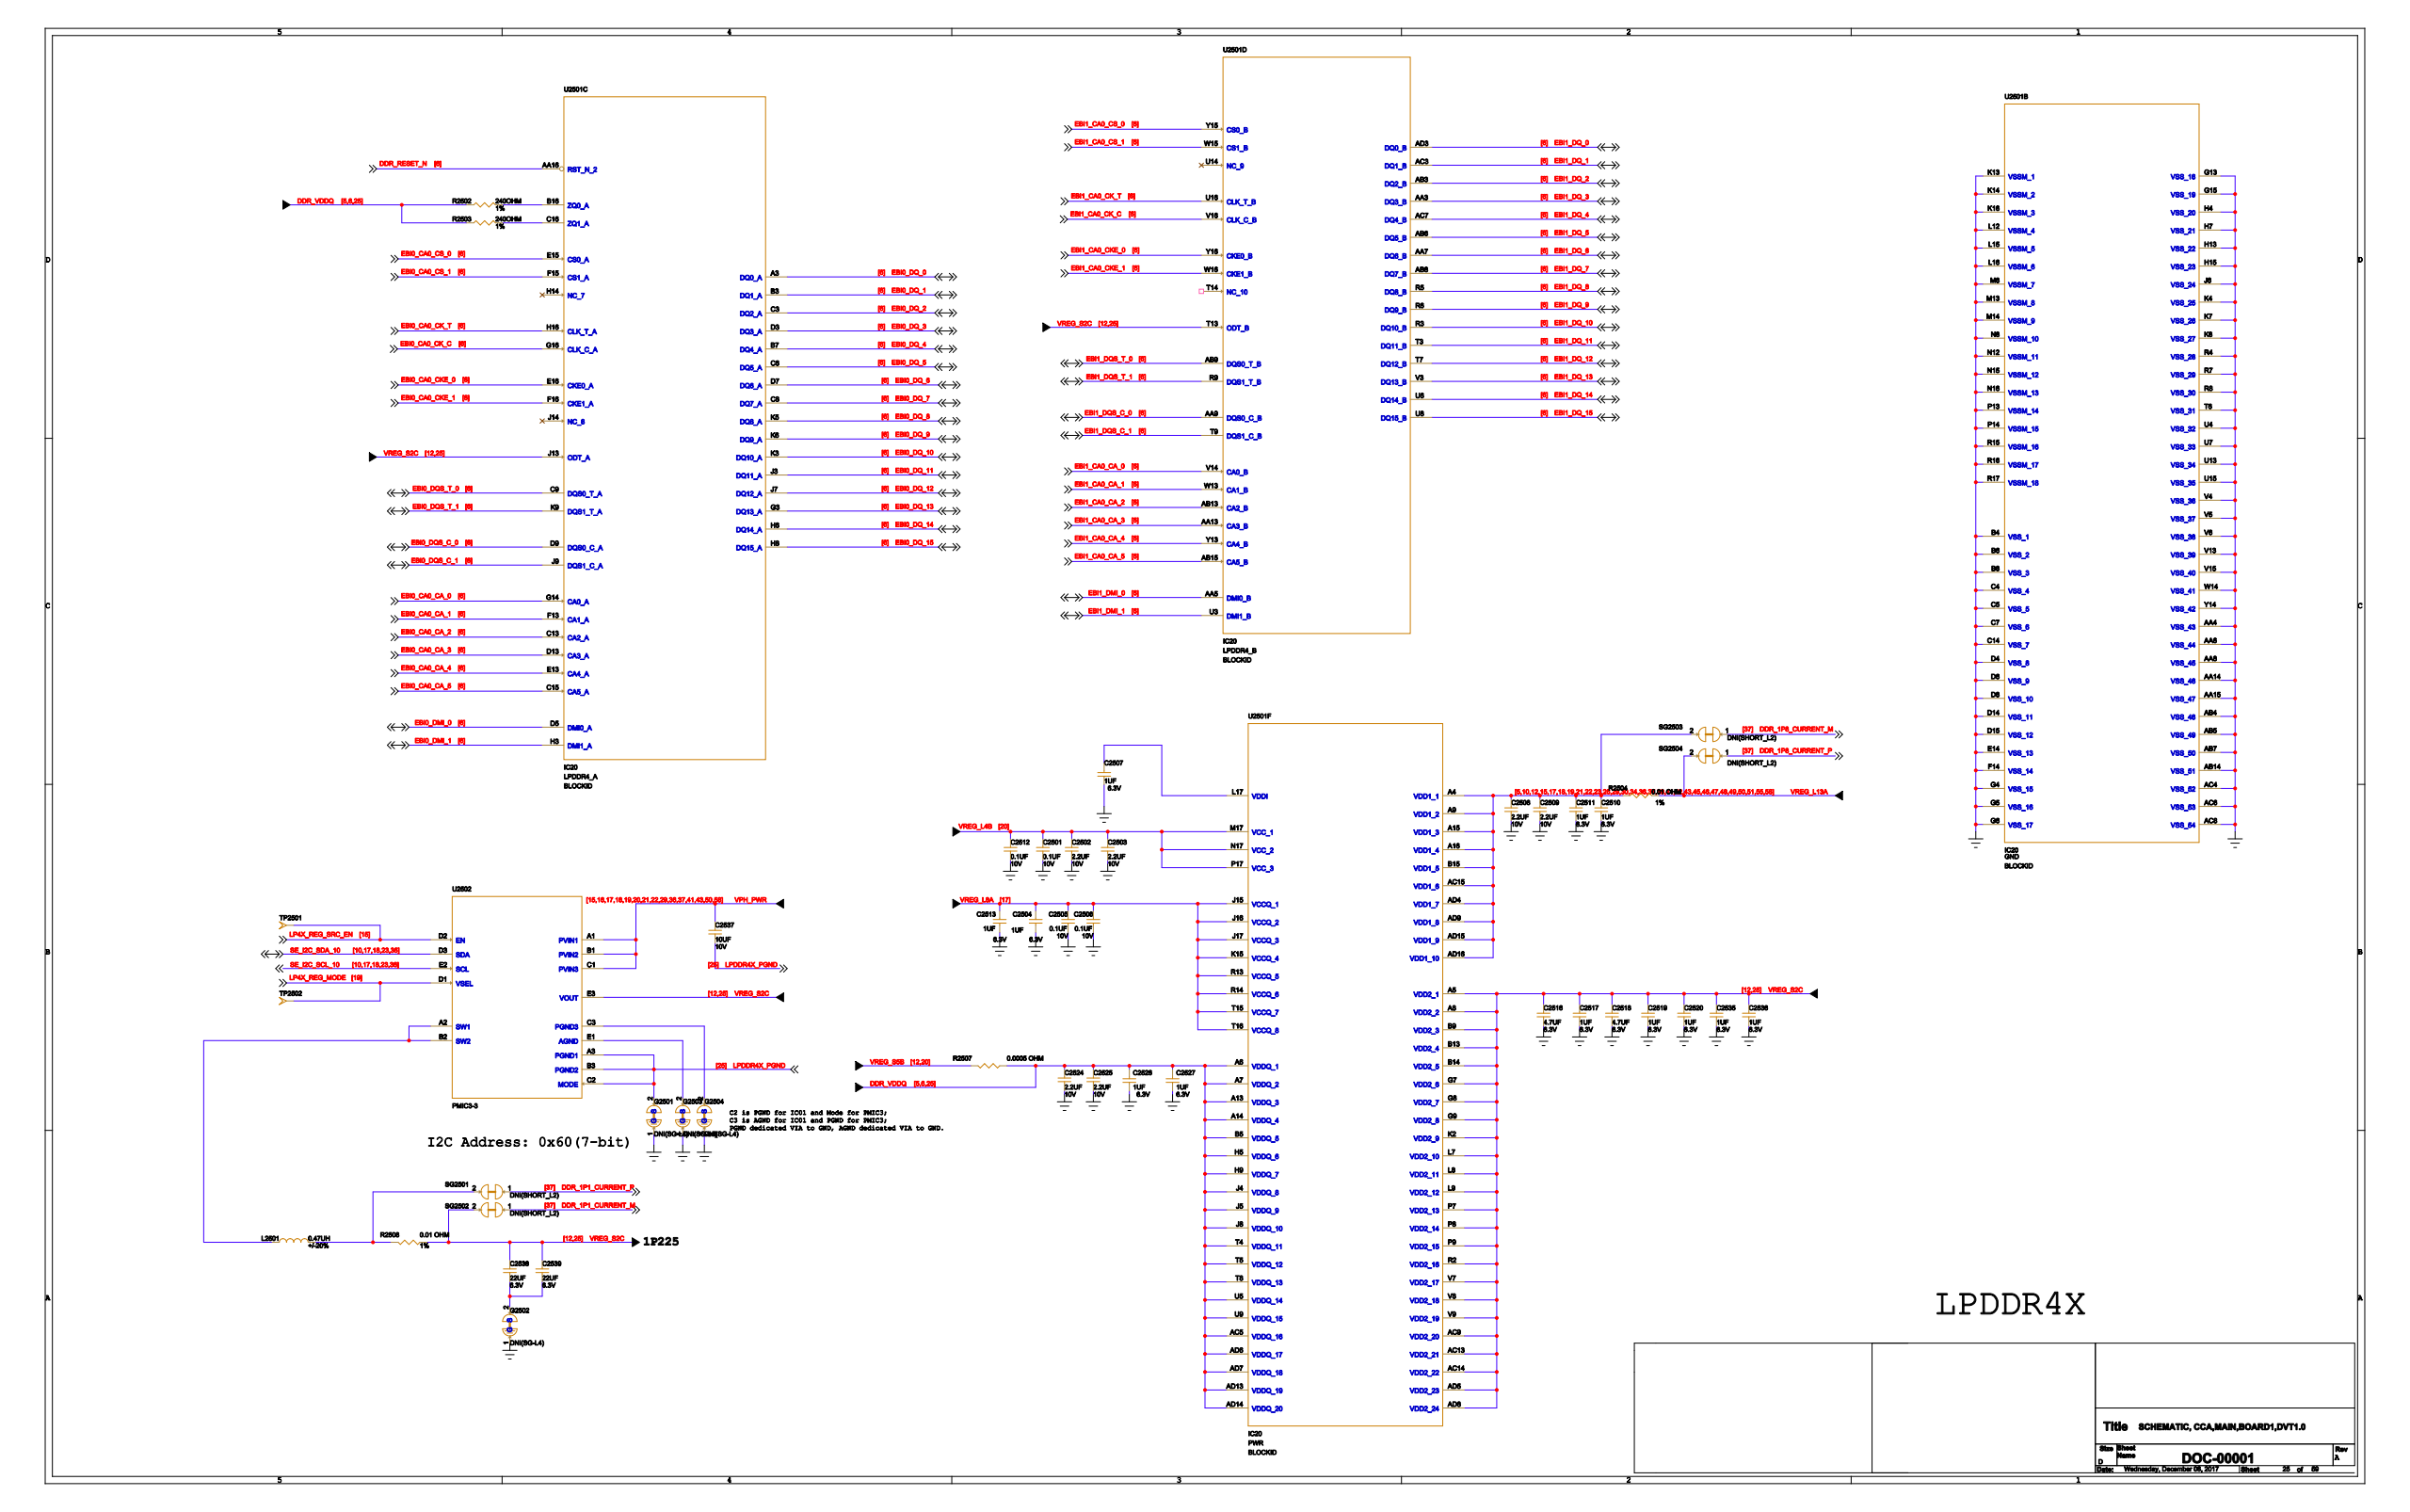Circuit board | KiCad | 1657 parts | 1365 nets | one sheet of the schematic
Parts on this sheet (reference | value | footprint):
C2501
C2502
C2503
C2504
C2505
C2506
C2507
C2508
C2509
C2510
C2511
C2512
C2513
C2516
C2517
C2518
C2519
C2520
C2524
C2525
C2526
C2527
C2535
C2536
C2537
C2538
C2539
G2501
G2502
G2503
G2504
L2501
R2502
R2503
R2504
R2507
R2508
SG2501
SG2502
SG2503
SG2504
TP2501
TP2502
U2501
U2502
Nets of these parts (net: part-pin ...):
DDR_VDDQ: C2524-1 C2525-1 C2526-2 C2527-2 R2502-1 R2503-1 R2507-2 U2501-A6 U2501-A7 U2501-A13 U2501-A14 U2501-AC5 U2501-AD6 U2501-AD7 U2501-AD13 U2501-AD14 U2501-B5 U2501-H5 U2501-H9 U2501-J4 U2501-J5 U2501-J8 U2501-T4 U2501-T5 U2501-T8 U2501-U5 U2501-U9
GND: C2501-2 C2502-2 C2503-2 C2504-2 C2505-2 C2506-2 C2507-1 C2508-2 C2509-2 C2510-2 C2511-2 C2512-2 C2513-2 C2516-2 C2517-2 C2518-2 C2519-2 C2520-2 C2524-2 C2525-2 C2526-1 C2527-1 C2535-2 C2536-2 G2501-1 G2502-1 G2503-1 G2504-1 U2501-AA4 U2501-AA6 U2501-AA8 U2501-AA14 U2501-AA15 U2501-AB4 U2501-AB5 U2501-AB7 U2501-AB14 U2501-AC4 U2501-AC6 U2501-AC8 U2501-B4 U2501-B6 U2501-B8 U2501-C4 U2501-C5 U2501-C7 U2501-C14 U2501-D4 U2501-D6 U2501-D8 U2501-D14 U2501-D15 U2501-E14 U2501-F14 U2501-G4 U2501-G5 U2501-G6 U2501-G13 U2501-G15 U2501-H4 U2501-H7 U2501-H13 U2501-H15 U2501-J6 U2501-K4 U2501-K7 U2501-K8 U2501-K13 U2501-K14 U2501-K16 U2501-L12 U2501-L15 U2501-L16 U2501-M8 U2501-M13 U2501-M14 U2501-N8 U2501-N12 U2501-N15 U2501-N16 U2501-P13 U2501-P14 U2501-R4 U2501-R7 U2501-R8 U2501-R15 U2501-R16 U2501-R17 U2501-T6 U2501-U4 U2501-U7 U2501-U13 U2501-U15 U2501-V4 U2501-V5 U2501-V6 U2501-V13 U2501-V15 U2501-W14 U2501-Y14
VREG_L13A: R2504-1 SG2504-2
VPH_PWR: C2537-1 U2502-A1 U2502-B1 U2502-C1
N23907455: C2508-1 C2509-1 C2510-1 C2511-1 R2504-2 SG2503-2 U2501-A4 U2501-A9 U2501-A15 U2501-A16 U2501-AC15 U2501-AD4 U2501-AD9 U2501-AD15 U2501-AD16 U2501-B15
SE_I2C_SCL_10: U2502-E2
SE_I2C_SDA_10: U2502-D3
VREG_S2C: C2516-1 C2517-1 C2518-1 C2519-1 C2520-1 C2535-1 C2536-1 C2538-1 C2539-1 R2508-2 SG2502-2 U2502-E3 U2501-A5 U2501-A8 U2501-AC9 U2501-AC13 U2501-AC14 U2501-AD5 U2501-AD8 U2501-B9 U2501-B13 U2501-B14 U2501-G7 U2501-G8 U2501-G9 U2501-J13 U2501-K2 U2501-L7 U2501-L8 U2501-L9 U2501-P7 U2501-P8 U2501-P9 U2501-R2 U2501-T13 U2501-V7 U2501-V8 U2501-V9
N23906069: R2503-2 U2501-C16
N23911865: C2538-2 C2539-2 G2502-2
_1P1_CURRENT_M: SG2502-1
N23907588: C2507-2 U2501-L17
N23911869: L2501-2 R2508-1 SG2501-2
N23907573: L2501-1 U2502-A2 U2502-B2
LPDDR4X_PGND: C2537-2 G2501-2 U2502-A3 U2502-B3 U2502-C2
N23907567: G2504-2 U2502-C3
LP4X_REG_MODE: TP2502-1 U2502-D1
P4X_REG_SRC_EN: TP2501-1 U2502-D2
N23907547: G2503-2 U2502-E1
VREG_L8A: C2504-1 C2505-1 C2506-1 C2513-1 U2501-J15 U2501-J16 U2501-J17 U2501-K15 U2501-R13 U2501-R14 U2501-T15 U2501-T16
EBI0_DQ_0: U2501-A3
EBI1_DQ_3: U2501-AA3
EBI1_DMI_0: U2501-AA5
EBI1_DQ_6: U2501-AA7
EBI1_DQS_C_0: U2501-AA9
EBI1_CA0_CA_3: U2501-AA13
DDR_RESET_N: U2501-AA16
EBI1_DQ_2: U2501-AB3
EBI1_DQ_5: U2501-AB6
EBI1_DQ_7: U2501-AB8
EBI1_DQS_T_0: U2501-AB9
EBI1_CA0_CA_2: U2501-AB13
EBI1_CA0_CA_5: U2501-AB15
EBI1_DQ_1: U2501-AC3
EBI1_DQ_4: U2501-AC7
EBI1_DQ_0: U2501-AD3
EBI0_DQ_1: U2501-B3
EBI0_DQ_4: U2501-B7
N23906067: R2502-2 U2501-B16
EBI0_DQ_2: U2501-C3
EBI0_DQ_5: U2501-C6
EBI0_DQ_7: U2501-C8
EBI0_DQS_T_0: U2501-C9
EBI0_CA0_CA_2: U2501-C13
EBI0_CA0_CA_5: U2501-C15
EBI0_DQ_3: U2501-D3
EBI0_DMI_0: U2501-D5
EBI0_DQ_6: U2501-D7
EBI0_DQS_C_0: U2501-D9
EBI0_CA0_CA_3: U2501-D13
EBI0_CA0_CA_4: U2501-E13
EBI0_CA0_CS_0: U2501-E15
EBI0_CA0_CKE_0: U2501-E16
EBI0_CA0_CA_1: U2501-F13
EBI0_CA0_CS_1: U2501-F15
EBI0_CA0_CKE_1: U2501-F16
EBI0_DQ_13: U2501-G3
EBI0_CA0_CA_0: U2501-G14
EBI0_CA0_CK_C: U2501-G16
EBI0_DMI_1: U2501-H3
EBI0_DQ_14: U2501-H6
EBI0_DQ_15: U2501-H8
EBI0_CA0_CK_T: U2501-H16
EBI0_DQ_11: U2501-J3
EBI0_DQ_12: U2501-J7
EBI0_DQS_C_1: U2501-J9
EBI0_DQ_10: U2501-K3
EBI0_DQ_8: U2501-K5
EBI0_DQ_9: U2501-K6
EBI0_DQS_T_1: U2501-K9
VREG_L4B: C2501-1 C2502-1 C2503-1 C2512-1 U2501-M17 U2501-N17 U2501-P17
EBI1_DQ_10: U2501-R3
EBI1_DQ_8: U2501-R5
EBI1_DQ_9: U2501-R6
EBI1_DQS_T_1: U2501-R9
EBI1_DQ_11: U2501-T3
EBI1_DQ_12: U2501-T7
EBI1_DQS_C_1: U2501-T9
EBI1_DMI_1: U2501-U3
EBI1_DQ_14: U2501-U6
EBI1_DQ_15: U2501-U8
EBI1_CA0_CK_T: U2501-U16
EBI1_DQ_13: U2501-V3
EBI1_CA0_CA_0: U2501-V14
EBI1_CA0_CK_C: U2501-V16
EBI1_CA0_CA_1: U2501-W13
EBI1_CA0_CS_1: U2501-W15
EBI1_CA0_CKE_1: U2501-W16
EBI1_CA0_CA_4: U2501-Y13
EBI1_CA0_CS_0: U2501-Y15
EBI1_CA0_CKE_0: U2501-Y16
_1P8_CURRENT_M: SG2503-1
_1P8_CURRENT_P: SG2504-1
VREG_S5B: R2507-1
_1P1_CURRENT_P: SG2501-1